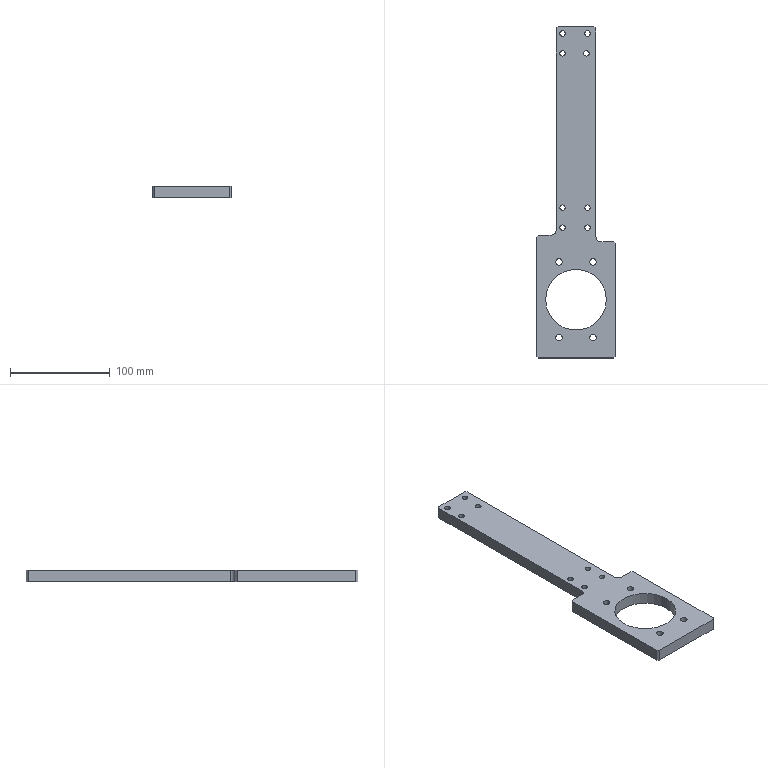Part | SolidWorks | features Chamfer 2, Cut 2, HoleWzd 2, Extrusion 1, Fillet 1 | 1 solid | 80 faces | box 80 x 333.5 x 12 mm | volume 174640 mm3 | cylinder 52 | plane 28 | commonest cylinder face diameters 10 x18 5.5 x16 6.6 x8 11 x8 61 x2